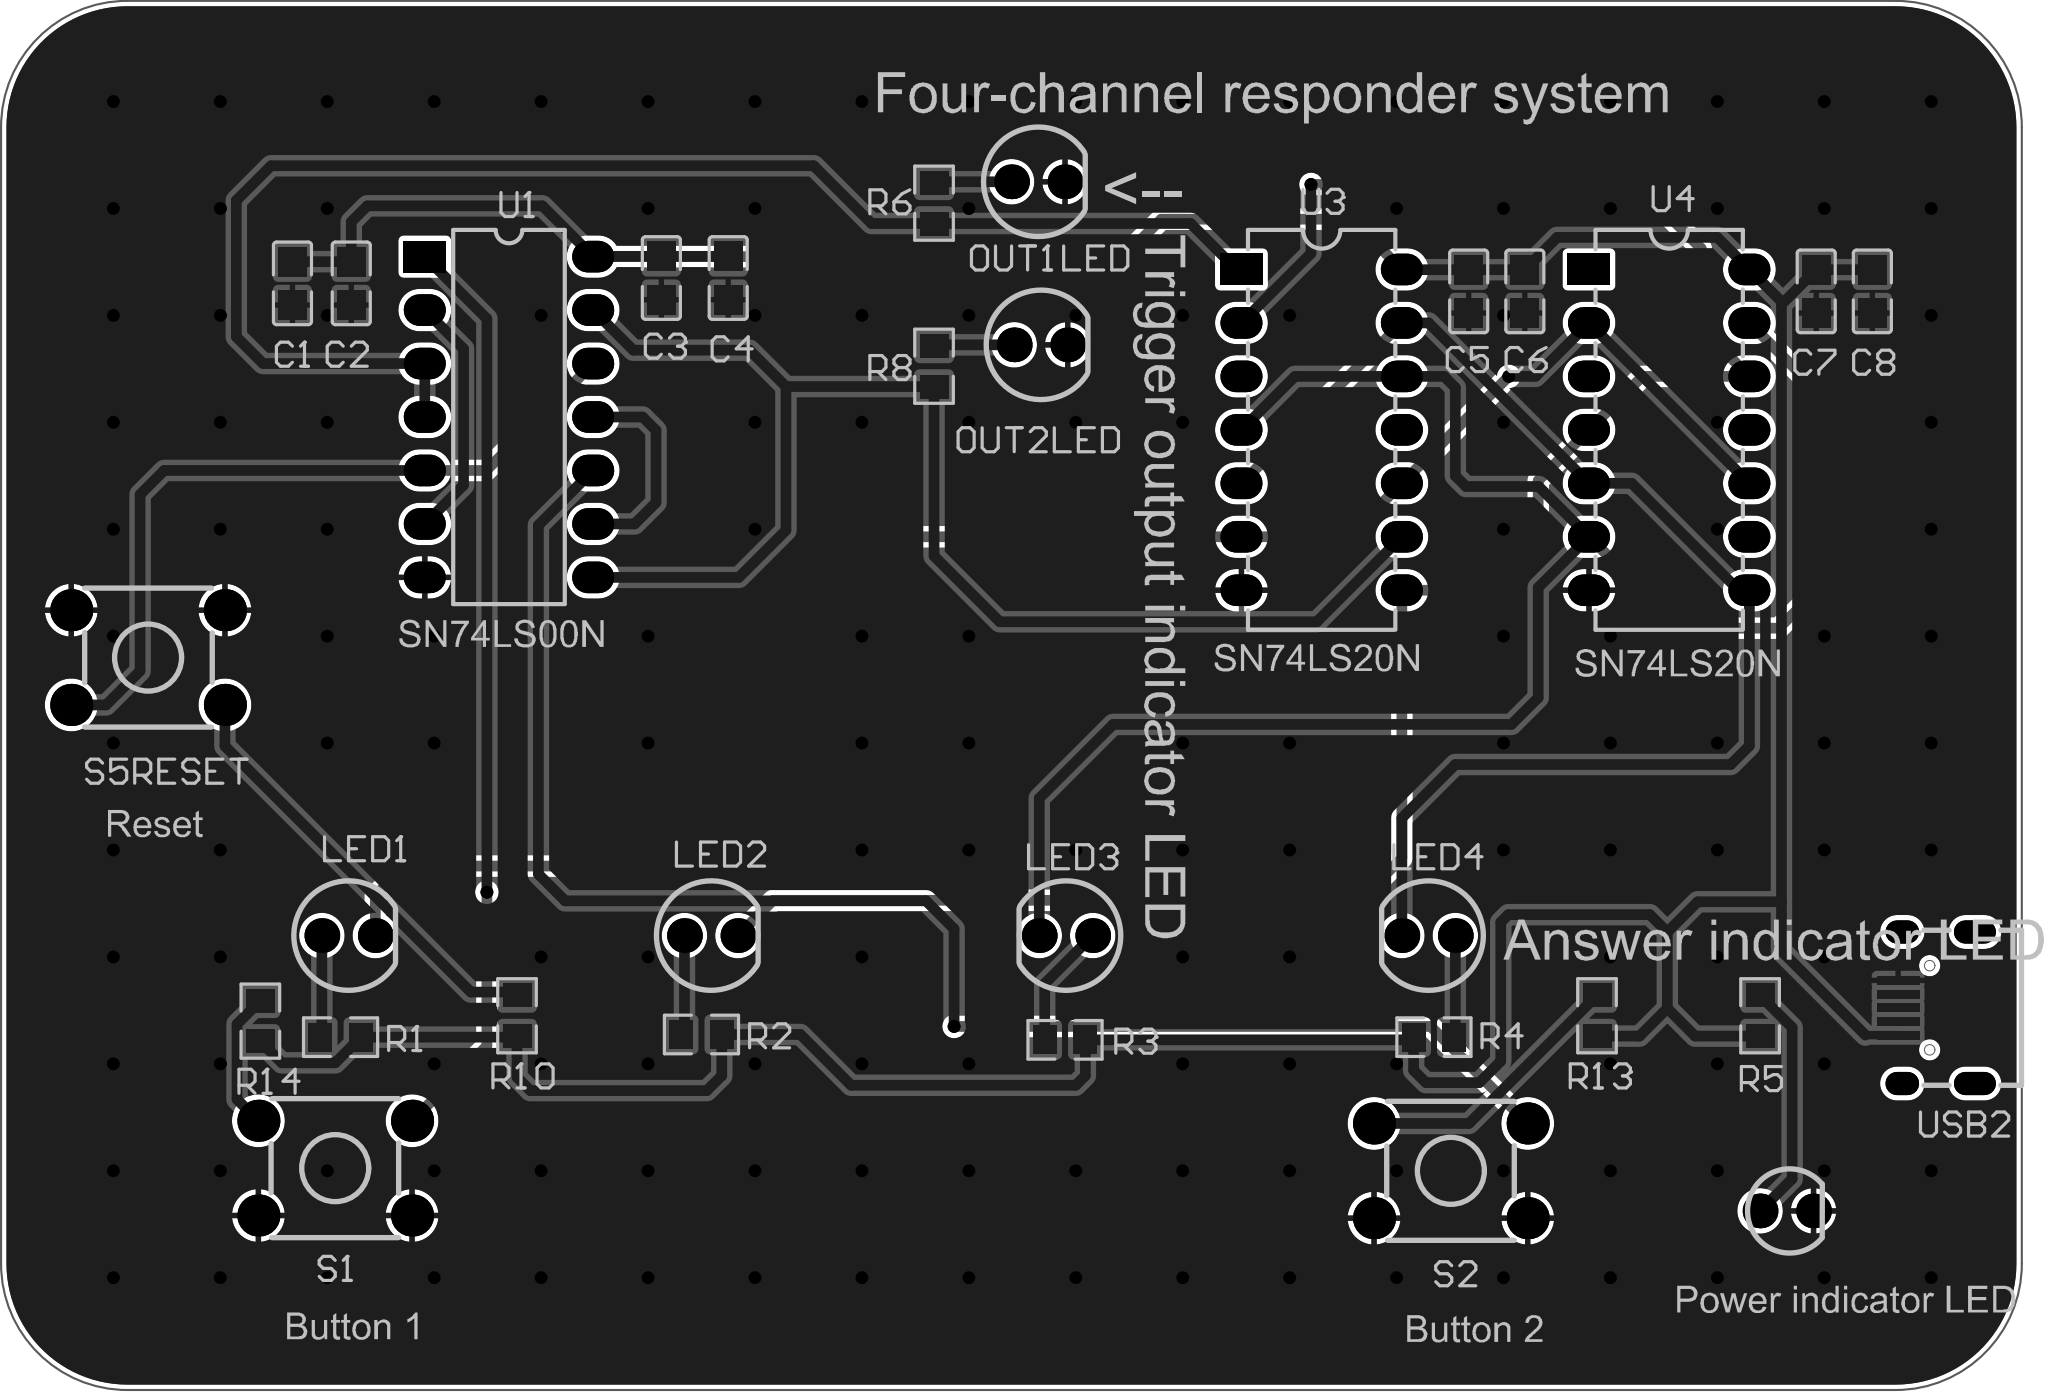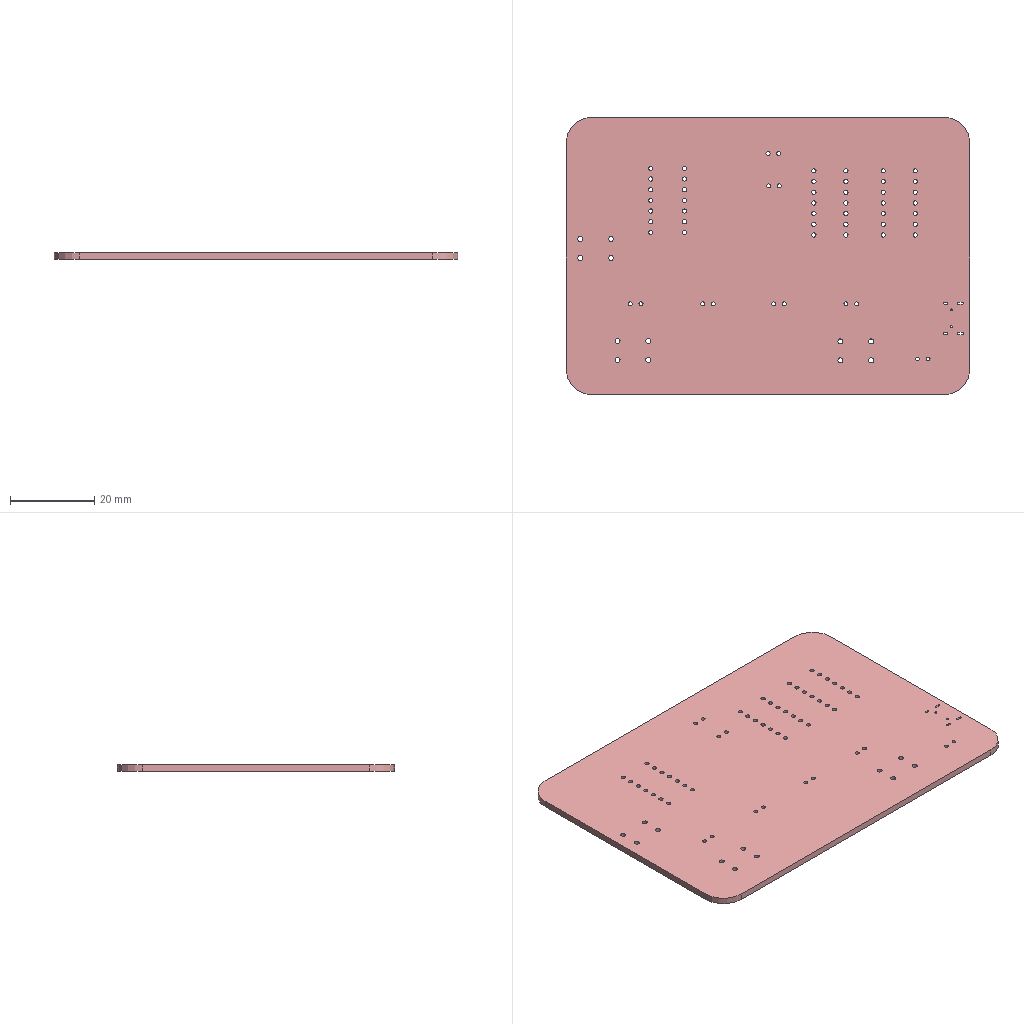Circuit board layout | Altium Designer | box 96 x 66 x 1.6 mm
Layer stack:
# Altium Designer layer stack of  (unit mm; dielectric type: 0 none, 1 core, 2 prepreg, 3 surface material)
index,name,kind,layer,copper_thickness_mm,dielectric_type,dielectric_thickness_mm,dielectric_material,dielectric_constant
0,Top Paste Mask Layer,other,,,,,,
1,Top Silkscreen Layer,other,,,,,,
2,Top Solder Mask Layer,dielectric,,,3,0.01,,3.3
3,Top Layer,copper,Top Layer,0.035,,,,
4,Dielectric1,dielectric,,,3,1.51,FR4,4.5
5,Bottom Layer,copper,Bottom Layer,0.035,,,,
6,Bottom Solder Mask Layer,dielectric,,,3,0.01,,3.3
7,Bottom Silkscreen Layer,other,,,,,,
8,Bottom Paste Mask Layer,other,,,,,,
# drill layer pairs: low layer,high layer
drill_pair,Top Layer,Bottom Layer
Part placement:
Designator,Comment,Layer,Footprint,Center-X(mm),Center-Y(mm),Rotation
C1,10u,TopLayer,C0805,93.472,132.334,270
C2,0.1u,TopLayer,C0805,96.266,132.334,270
C3,10u,TopLayer,C0805,110.998,132.588,270
C4,0.1u,TopLayer,C0805,114.173,132.588,270
C5,10u,TopLayer,C0805,149.352,131.953,270
C6,0.1u,TopLayer,C0805,152.019,131.953,270
C7,10u,TopLayer,C0805,165.862,131.953,270
C8,0.1u,TopLayer,C0805,168.529,131.953,270
LED2,LED-TH-5mm_R,TopLayer,LED-TH_BD5.0_RED,113.365,101.346,90
LED3,LED-TH-5mm_R,TopLayer,LED-TH_BD5.0_RED,130.221,101.346,270
LED4,LED-TH-5mm_R,TopLayer,LED-TH_BD5.0_RED,147.447,101.346,270
OUT1LED,LED-TH-5mm_R,TopLayer,LED-TH_BD5.0_RED,128.905,137.16,90
OUT2LED,LED-TH-5mm_R,TopLayer,LED-TH_BD5.0_RED,129.032,129.413,90
R2,1k,TopLayer,R0805,112.903,96.647,0
R3,1k,TopLayer,R0805,130.175,96.393,0
R4,1k,TopLayer,R0805,147.701,96.52,180
R5,1k,TopLayer,R0805,163.195,97.536,90
R6,1k,TopLayer,R0805,123.952,136.144,90
R8,1k,TopLayer,R0805,123.952,128.397,90
R10,1k,TopLayer,R0805,104.14,97.536,90
R13,1k,TopLayer,R0805,155.448,97.536,90
R14,1k,TopLayer,R0805,91.948,97.282,90
S1,TC-1157-B-A,TopLayer,KEY-TH_4P-L6.4-W6.0-P4.50-LS7.3-TL,95.504,90.297,0
S2,TC-1157-B-A,TopLayer,KEY-TH_4P-L6.4-W6.0-P4.50-LS7.3-TL,148.505,90.17,0
U4,SN74LS20N,TopLayer,DIP-14_L19.0-W7.0-P2.54-LS7.6-BL,158.877,125.374,270
S5RESET,TC-1157-B-A,TopLayer,KEY-TH_4P-L6.4-W6.0-P4.50-LS7.3-TL,86.614,114.554,180
LED1,LED-TH-5mm_R,TopLayer,LED-TH_BD5.0_RED,96.139,101.346,90
LED5,LED-TH-3mm_R,TopLayer,LED-TH_BD3.0_RED,164.465,88.265,90
R1,1k,TopLayer,R0805,95.758,96.52,0
U1,SN74LS00N,TopLayer,PDIP-14_L19.7-W6.6-P2.54-LS8.3-BL,103.759,125.984,270
U3,SN74LS20N,TopLayer,DIP-14_L19.0-W7.0-P2.54-LS7.6-BL,142.367,125.374,270
USB2,U-F-M5DD-W-2-SUS,TopLayer,MICRO-USB-SMD_U-F-M5DD-W-2-SUS,171.577,97.917,270
Pad and via stacks:
# Altium Designer via and pad stacks of  (unit mm). Each distinct definition once, with the count of objects using it.
# via: kind,start_layer,end_layer,hole_mm,diameter_mm,mode(0 simple;1 top-mid-bottom;2 full stack),diameter_per_layer,count,example_net
# pad: kind,layer,hole_mm,hole_type(0 round;1 square;2 slot),plating,top_size,top_shape(1 round;2 rect;3 octagon;9 rounded rect),mid_size,bottom_size,mode,footprint,size_per_layer,count,example
pad,Top Layer,0,0,plated,1.41x1.35,2,1.41x1.35,1.41x1.35,0,C0805,,16,C1.2
pad,Top Layer,0,0,plated,1.133x1.377,2,1.133x1.377,1.133x1.377,0,R0805,,20,R2.2
pad,Top Layer,0,0,plated,0.4x2,2,0.4x2,0.4x2,0,MICRO-USB-SMD_U-F-M5DD-W-2-SUS,,5,USB2.1
pad,Multi-Layer,0.9652,0,plated,1.651x1.651,1,1.651x1.651,1.651x1.651,0,LED-TH_BD5.0_RED,,12,LED2.1
pad,Multi-Layer,1.2,0,plated,2x2,1,2x2,2x2,0,KEY-TH_4P-L6.4-W6.0-P4.50-LS7.3-TL,,12,S1.1
pad,Multi-Layer,1,0,plated,2x1.5,1,2x1.5,2x1.5,0,DIP-14_L19.0-W7.0-P2.54-LS7.6-BL,,26,U4.8
pad,Multi-Layer,1,0,plated,2x1.5,2,2x1.5,2x1.5,0,DIP-14_L19.0-W7.0-P2.54-LS7.6-BL,,2,U4.1
pad,Multi-Layer,0.9,0,plated,1.651x1.651,1,1.651x1.651,1.651x1.651,0,LED-TH_BD3.0_RED,,2,LED5.1
pad,Multi-Layer,1,0,plated,2x1.5,2,2x1.5,2x1.5,0,PDIP-14_L19.7-W6.6-P2.54-LS8.3-BL,,1,U1.1
pad,Multi-Layer,1,0,plated,2x1.5,1,2x1.5,2x1.5,0,PDIP-14_L19.7-W6.6-P2.54-LS8.3-BL,,13,U1.2
pad,Multi-Layer,0.5,2,plated,1.1x1.6,1,1.1x1.6,1.1x1.6,0,MICRO-USB-SMD_U-F-M5DD-W-2-SUS,,2,USB2.6
pad,Multi-Layer,0.5,2,plated,1.1x2,1,1.1x2,1.1x2,0,MICRO-USB-SMD_U-F-M5DD-W-2-SUS,,2,USB2.7
via,Top Layer,Bottom Layer,0.3048,0.6096,0,,159,S1
Copper pours:
name,layer,net,type(0 solid;1 hatched;2 none)
Bottom Layer-GND,Bottom Layer,GND,0
Top Layer-GND,Top Layer,GND,0
Design rules, without the lines most boards share:
# Altium Designer design rules of  (exported by Altium Designer, unit mm)
# columns: name | kind | enabled | priority | scope1 | scope2 | descriptor | typed fields (field=value)
Plane_innerPlane | 0 | disabled | 1 | All | All | Clearance Constraint (Gap=6mil) (Disabled)(All),(All) | gap=0.1524
Plane_innerPlane_1 | 63 | disabled | 1 | All | All | Board Clearance Constraint (Gap=0mil) (Disabled)(All) |
Copper_copperRegion | 0 | disabled | 2 | All | All | Clearance Constraint (Gap=6mil) (Disabled)(All),(All) | gap=0.1524
Copper_copperRegion_1 | 63 | disabled | 2 | All | All | Board Clearance Constraint (Gap=0mil) (Disabled)(All) |
Copper_gge8956 | 0 | disabled | 3 | All | All | Clearance Constraint (Gap=6mil) (Disabled)(All),(All) | gap=0.1524
Copper_gge8956_1 | 63 | disabled | 3 | All | All | Board Clearance Constraint (Gap=0mil) (Disabled)(All) |
Copper_gge8950 | 0 | disabled | 4 | All | All | Clearance Constraint (Gap=6mil) (Disabled)(All),(All) | gap=0.1524
Copper_gge8950_1 | 63 | disabled | 4 | All | All | Board Clearance Constraint (Gap=0mil) (Disabled)(All) |
safeClearance | 0 | enabled | 5 | All | All | Clearance Constraint (Gap=6mil) (All),(All) | gap=0.1524
safeClearance_1 | 63 | enabled | 5 | All | All | Board Clearance Constraint (Gap=0mil) (All) |
gge8956 | 52 | disabled | 1 | All | All | Hole To Hole Clearance (Gap=0mil) (Disabled)(All),(All) | gap=0
gge8950 | 52 | disabled | 2 | All | All | Hole To Hole Clearance (Gap=0mil) (Disabled)(All),(All) | gap=0
Common | 52 | enabled | 3 | All | All | Hole To Hole Clearance (Gap=11.8mil) (All),(All) | gap=0.2997
trackWidth | 2 | enabled | 1 | All | All | Width Constraint (Min=5mil) (Max=100mil) (Preferred=20mil) (All) |
viaSize | 11 | enabled | 1 | All | All | Routing Via (MinHoleWidth=11.8mil) (MaxHoleWidth=236.2mil) (PreferredHoleWidth=12mil) (MinWidth=19.7mil) (MaxWidth=393.7mil) (PreferedWidth=24mil) (All) | via_min_hole=0.2997 via_max_hole=6 via_preferred_diameter=0.6096 via_preferred_hole=0.3048
gge8956_1 | 20 | disabled | 1 | All | All | Polygon Connect Rule(Relief Connect )(Conductor Width=10mil) (Relief Angle=90 Angle) (Entries=4) (Air Gap Width=10mil) (Disabled)(All),(All) | connect_style(0=relief,1=direct,2=none)=0 relief_conductor_width=0.254 relief_entries=4
gge8950_1 | 20 | disabled | 2 | All | All | Polygon Connect Rule(Relief Connect )(Conductor Width=10mil) (Relief Angle=90 Angle) (Entries=4) (Air Gap Width=10mil) (Disabled)(All),(All) | connect_style(0=relief,1=direct,2=none)=0 relief_conductor_width=0.254 relief_entries=4
copperRegion | 20 | enabled | 3 | All | All | Polygon Connect Rule(Relief Connect )(Conductor Width=10mil) (Relief Angle=90 Angle) (Entries=4) (Air Gap Width=10mil) (All),(All) | connect_style(0=relief,1=direct,2=none)=0 relief_conductor_width=0.254 relief_entries=4